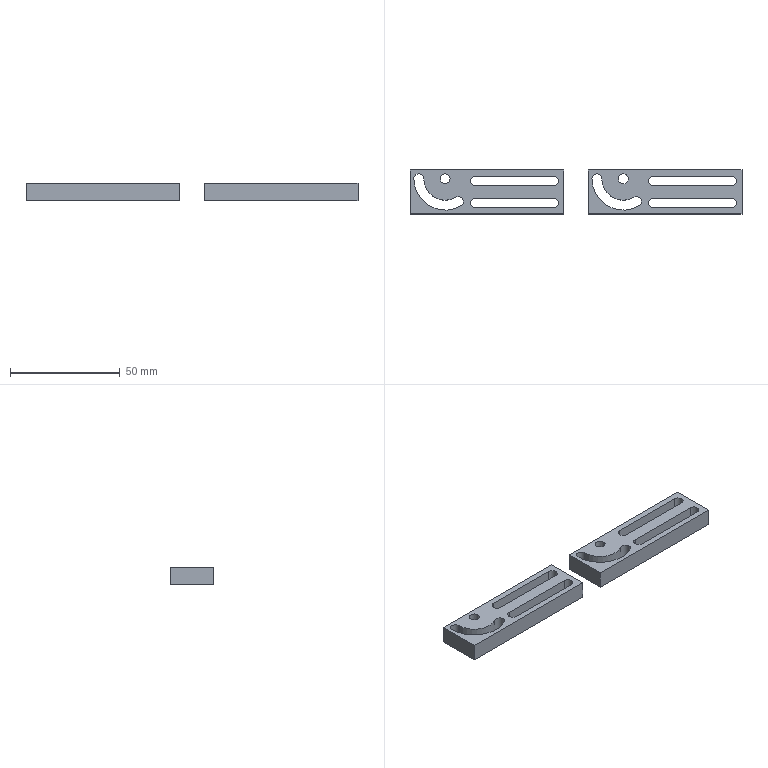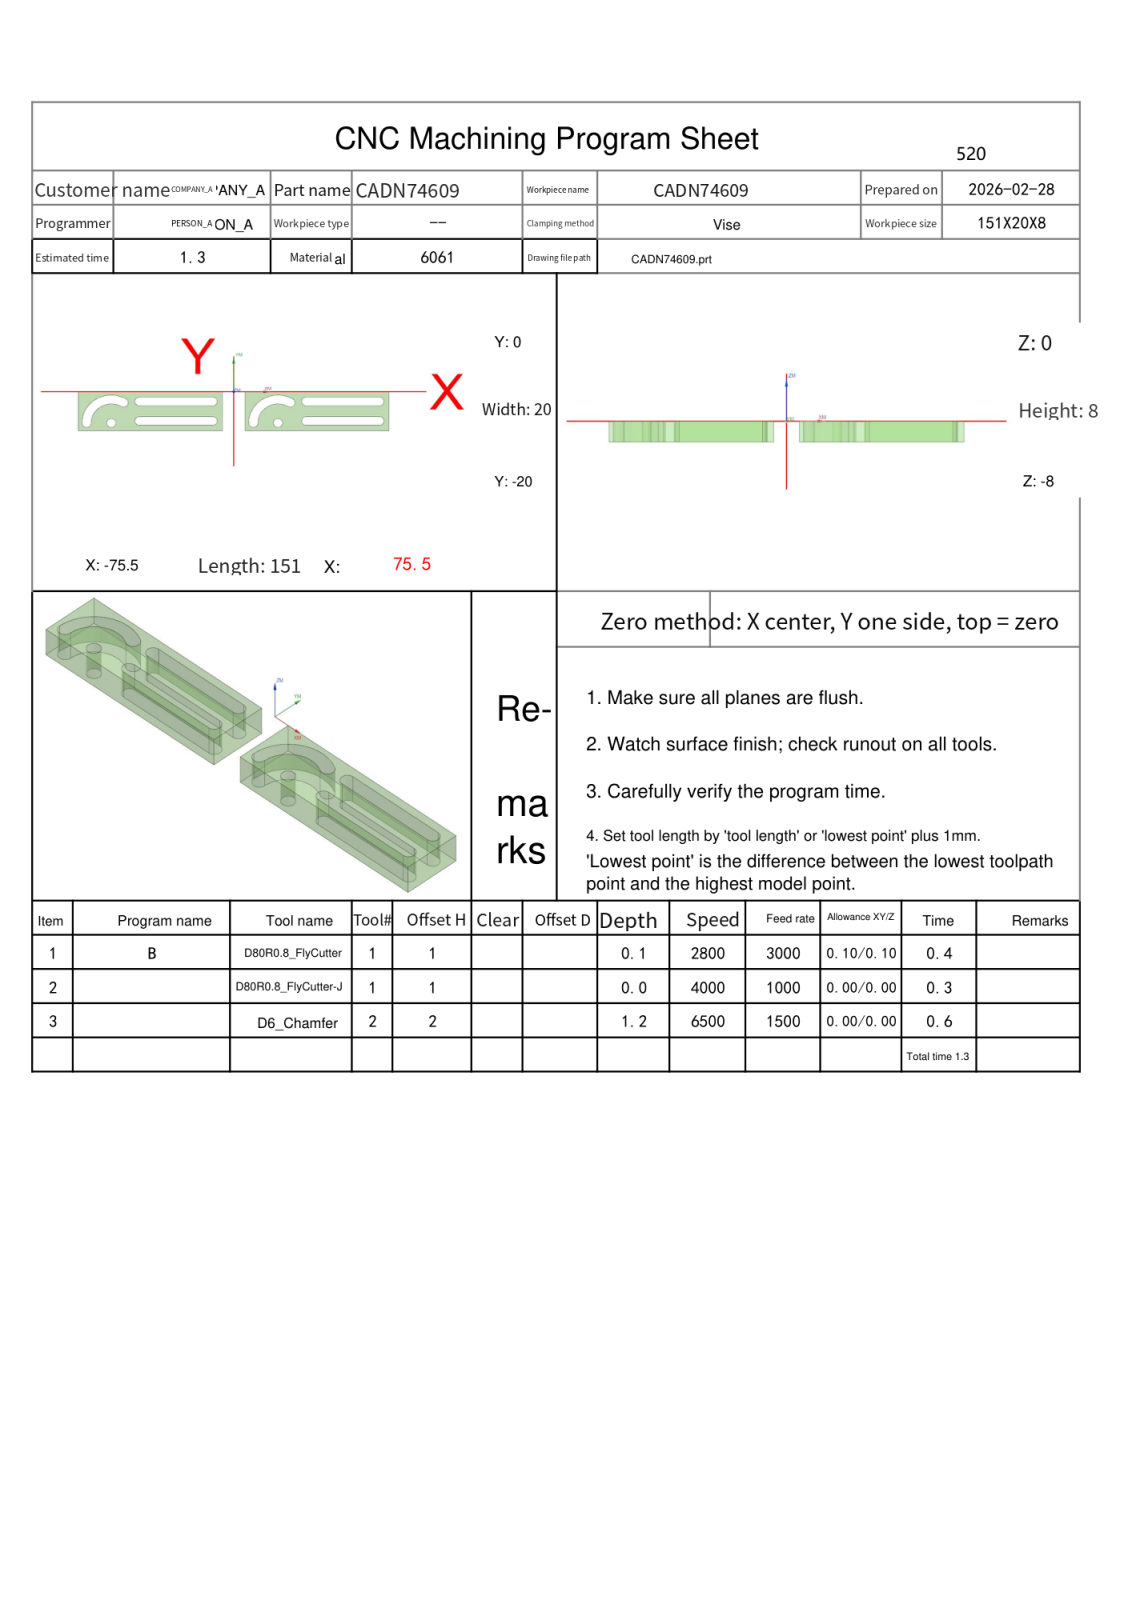NC program | NX | posted by the shop | part box 151 x 20 x 8 mm
Whole program:
%
O0001
(Machine time: 1.91 MIN)
(===Total Tool:2===)
(T1=D80R0.8-FlyCutter D=80.  R=0.8  D-  H01 Z=0.    )
(T2=D6_Chamfer   D=6.   R=0.   D-  H02 Z=-1.2  )
G80 G90 G17 G49 G40
G91 G28 Z0
M01
N1 T01 M06
(D80R0.8-FlyCutter  D=80. R=0.8 H=01 ce=0.10 di=0.10)
G00 G90 G54 X127.597 Y-10. M03 S2800
G43 H01 Z50.
M08
Z3.525
G01 Z1.525 F3000.
X115.597
X-115.597
X-127.597
Z3.525
G00 X127.597
Z3.05
G01 Z1.05
X115.597
X-115.597
X-127.597
Z3.05
G00 X127.597
Z2.575
G01 Z.575
X115.597
X-115.597
X-127.597
Z2.575
G00 X127.597
Z2.1
G01 Z.1
X115.597
X-115.597
X-127.597
Z2.1
G00 Z50.
G91 G28 Z0.0
M05
M09
G91 G28 Z0.0
M01
N2 T01 M06
(D80R0.8-FlyCutter-J  D=80. R=0.8 H=01 ce=0.00 di=0.00)
G00 G90 G54 X127.499 Y-10. M03 S4000
G43 H01 Z50.
M08
Z2.
G01 Z0.0 F1000.
X115.499
X-115.499
X-127.499
Z2.
G00 Z50.
G91 G28 Z0.0
M05
M09
G91 G28 Z0.0
M01
N3 T02 M06
(D6_Chamfer  D=6. R=0. H=02 ce=0.00 di=0.00)
G00 G90 G54 X40.886 Y-21.227 M03 S6500
G43 H02 Z50.
M08
Z.172
G01 Z-1.2 F1500.
G03 X40.6 Y-21.027 I-1.286 J-1.532
G01 X40.554 Y-20.997
X40.5 Y-21.
X5.5
G02 X4.5 Y-20. I0.0 J1.
G01 Y0.0
G02 X5.5 Y1. I1. J0.0
G01 X75.5
G02 X76.5 Y0.0 I0.0 J-1.
G01 Y-20.
G02 X75.5 Y-21. I-1. J0.0
G01 X40.5
X40.446 Y-20.997
X40.4 Y-21.027
G03 X40.114 Y-21.227 I1. J-1.732
G01 Z.172
G00 Z10.
X15.322 Y-4.512
Z.202
G01 Z-1.2
G03 X15.049 Y-4.493 I-.273 J-1.981
G01 X14.974 Y-4.495
X14.92 Y-4.494
X14.875 Y-4.525
G03 X8.25 Y-16. I6.625 J-11.475
X9.5 Y-17.25 I1.25 J0.0
X10.75 Y-16. I0.0 J1.25
G02 X21.5 Y-5.25 I10.75 J0.0
X26.875 Y-6.69 I0.0 J-10.75
G03 X27.5 Y-6.858 I.625 J1.083
X28.75 Y-5.608 I0.0 J1.25
X28.125 Y-4.525 I-1.25 J0.0
X21.5 Y-2.75 I-6.625 J-11.475
X14.875 Y-4.525 I0.0 J-13.25
G01 X14.826 Y-4.548
X14.799 Y-4.596
G03 X14.64 Y-4.906 I1.693 J-1.064
G01 Z.202
G00 Z10.
X22.565 Y-16.407
Z.294
G01 Z-1.2
G03 X22.734 Y-16.102 I-1.658 J1.118
G01 X22.759 Y-16.054
X22.75 Y-16.
G03 X21.5 Y-14.75 I-1.25 J0.0
X20.25 Y-16. I0.0 J-1.25
X21.5 Y-17.25 I1.25 J0.0
X22.723 Y-16.26 I0.0 J1.25
G01 X22.75 Y-16.
X22.759 Y-15.946
X22.734 Y-15.898
G03 X22.565 Y-15.593 I-1.827 J-.813
G01 Z.294
G00 Z10.
X52.614 Y-16.023
Z.172
G01 Z-1.2
G03 X52.9 Y-16.223 I1.286 J1.532
G01 X52.946 Y-16.253
X53. Y-16.25
X70.75
G03 X72. Y-15. I0.0 J1.25
X70.75 Y-13.75 I-1.25 J0.0
G01 X35.25
G03 X34. Y-15. I0.0 J-1.25
X35.25 Y-16.25 I1.25 J0.0
G01 X53.
X53.054 Y-16.253
X53.1 Y-16.223
G03 X53.386 Y-16.023 I-1. J1.732
G01 Z.172
G00 Z2.55
X52.614 Y-6.023
Z.172
G01 Z-1.2
G03 X52.9 Y-6.223 I1.286 J1.532
G01 X52.946 Y-6.253
X53. Y-6.25
X70.75
G03 X72. Y-5. I0.0 J1.25
X70.75 Y-3.75 I-1.25 J0.0
G01 X35.25
G03 X34. Y-5. I0.0 J-1.25
X35.25 Y-6.25 I1.25 J0.0
G01 X53.
X53.054 Y-6.253
X53.1 Y-6.223
G03 X53.386 Y-6.023 I-1. J1.732
G01 Z.172
G00 Z10.
X-40.886 Y1.227
Z.172
G01 Z-1.2
G03 X-40.6 Y1.027 I1.286 J1.532
G01 X-40.554 Y.997
X-40.5 Y1.
X-5.5
G02 X-4.5 Y0.0 I0.0 J-1.
G01 Y-20.
G02 X-5.5 Y-21. I-1. J0.0
G01 X-75.5
G02 X-76.5 Y-20. I0.0 J1.
G01 Y0.0
G02 X-75.5 Y1. I1. J0.0
G01 X-40.5
X-40.446 Y.997
X-40.4 Y1.027
G03 X-40.114 Y1.227 I-1. J1.732
G01 Z.172
G00 Z10.
X-65.678 Y-4.512
Z.202
G01 Z-1.2
G03 X-65.951 Y-4.493 I-.273 J-1.981
G01 X-66.026 Y-4.495
X-66.08 Y-4.494
X-66.125 Y-4.525
G03 X-72.75 Y-16. I6.625 J-11.475
X-71.5 Y-17.25 I1.25 J0.0
X-70.25 Y-16. I0.0 J1.25
G02 X-59.5 Y-5.25 I10.75 J0.0
X-54.125 Y-6.69 I0.0 J-10.75
G03 X-53.5 Y-6.858 I.625 J1.083
X-52.25 Y-5.608 I0.0 J1.25
X-52.875 Y-4.525 I-1.25 J0.0
X-59.5 Y-2.75 I-6.625 J-11.475
X-66.125 Y-4.525 I0.0 J-13.25
G01 X-66.174 Y-4.548
X-66.201 Y-4.596
G03 X-66.36 Y-4.906 I1.693 J-1.064
G01 Z.202
G00 Z10.
X-58.435 Y-16.407
Z.294
G01 Z-1.2
G03 X-58.266 Y-16.102 I-1.658 J1.118
G01 X-58.241 Y-16.054
X-58.25 Y-16.
G03 X-59.5 Y-14.75 I-1.25 J0.0
X-60.75 Y-16. I0.0 J-1.25
X-59.5 Y-17.25 I1.25 J0.0
X-58.277 Y-16.26 I0.0 J1.25
G01 X-58.25 Y-16.
X-58.241 Y-15.946
X-58.266 Y-15.898
G03 X-58.435 Y-15.593 I-1.827 J-.813
G01 Z.294
G00 Z10.
X-28.386 Y-16.023
Z.172
G01 Z-1.2
G03 X-28.1 Y-16.223 I1.286 J1.532
G01 X-28.054 Y-16.253
X-28. Y-16.25
X-10.25
G03 X-9. Y-15. I0.0 J1.25
X-10.25 Y-13.75 I-1.25 J0.0
G01 X-45.75
G03 X-47. Y-15. I0.0 J-1.25
X-45.75 Y-16.25 I1.25 J0.0
G01 X-28.
X-27.946 Y-16.253
X-27.9 Y-16.223
G03 X-27.614 Y-16.023 I-1. J1.732
G01 Z.172
G00 Z2.55
X-28.386 Y-6.023
Z.172
G01 Z-1.2
G03 X-28.1 Y-6.223 I1.286 J1.532
G01 X-28.054 Y-6.253
X-28. Y-6.25
X-10.25
G03 X-9. Y-5. I0.0 J1.25
X-10.25 Y-3.75 I-1.25 J0.0
G01 X-45.75
G03 X-47. Y-5. I0.0 J-1.25
X-45.75 Y-6.25 I1.25 J0.0
G01 X-28.
X-27.946 Y-6.253
X-27.9 Y-6.223
G03 X-27.614 Y-6.023 I-1. J1.732
G01 Z.172
G00 Z50.
M05
M09
G91 G28 Z0.0
G91 G28 Y0.0
M30
%